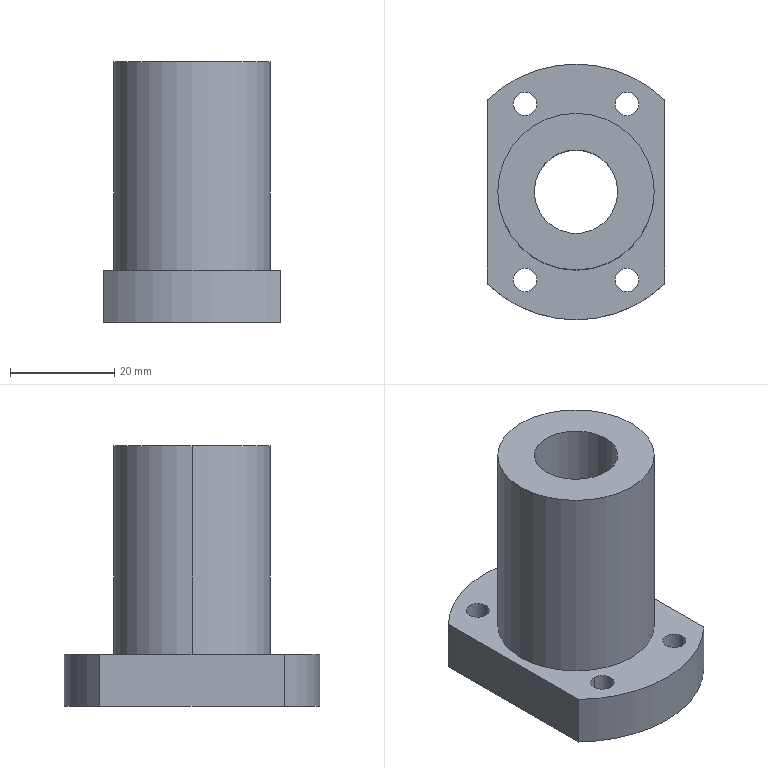Part | STEP file | SFI1605-4 | 2 solids | 34 faces | box 34 x 49 x 50 mm | volume 32157 mm3 | cylinder 24 | plane 10 | commonest cylinder face diameters 4.5 x8 8 x8 16 x4 30 x2 49 x2
STEP:
#1=CARTESIAN_POINT('',(8.,0.,523.5));
#2=VERTEX_POINT('',#1);
#3=CARTESIAN_POINT('',(-8.,0.,523.5));
#4=VERTEX_POINT('',#3);
#5=CARTESIAN_POINT('',(0.,0.,523.5));
#6=DIRECTION('',(0.,0.,-1.));
#7=DIRECTION('',(1.,0.,0.));
#8=AXIS2_PLACEMENT_3D('',#5,#6,#7);
#9=CIRCLE('',#8,8.);
#10=EDGE_CURVE('',#2,#4,#9,.T.);
#11=ORIENTED_EDGE('',*,*,#10,.F.);
#12=CARTESIAN_POINT('',(8.,0.,483.5));
#13=VERTEX_POINT('',#12);
#14=CARTESIAN_POINT('',(8.,0.,523.5));
#15=DIRECTION('',(0.,0.,-1.));
#16=VECTOR('',#15,1000.);
#17=LINE('',#14,#16);
#18=EDGE_CURVE('',#2,#13,#17,.T.);
#19=ORIENTED_EDGE('',*,*,#18,.T.);
#20=CARTESIAN_POINT('',(-8.,0.,483.5));
#21=VERTEX_POINT('',#20);
#22=CARTESIAN_POINT('',(0.,0.,483.5));
#23=DIRECTION('',(0.,0.,1.));
#24=DIRECTION('',(1.,0.,0.));
#25=AXIS2_PLACEMENT_3D('',#22,#23,#24);
#26=CIRCLE('',#25,8.);
#27=EDGE_CURVE('',#21,#13,#26,.T.);
#28=ORIENTED_EDGE('',*,*,#27,.F.);
#29=CARTESIAN_POINT('',(-8.,0.,523.5));
#30=DIRECTION('',(0.,0.,-1.));
#31=VECTOR('',#30,1000.);
#32=LINE('',#29,#31);
#33=EDGE_CURVE('',#4,#21,#32,.T.);
#34=ORIENTED_EDGE('',*,*,#33,.F.);
#35=EDGE_LOOP('',(#11,#19,#28,#34));
#36=FACE_OUTER_BOUND('',#35,.T.);
#37=CARTESIAN_POINT('',(0.,0.,523.5));
#38=DIRECTION('',(0.,0.,-1.));
#39=DIRECTION('',(-1.,0.,0.));
#40=AXIS2_PLACEMENT_3D('',#37,#38,#39);
#41=CYLINDRICAL_SURFACE('',#40,8.);
#42=ADVANCED_FACE('',(#36),#41,.F.);
#43=CARTESIAN_POINT('',(-15.,0.,523.5));
#44=VERTEX_POINT('',#43);
#45=CARTESIAN_POINT('',(15.,0.,523.5));
#46=VERTEX_POINT('',#45);
#47=CARTESIAN_POINT('',(0.,0.,523.5));
#48=DIRECTION('',(0.,0.,-1.));
#49=DIRECTION('',(-1.,0.,0.));
#50=AXIS2_PLACEMENT_3D('',#47,#48,#49);
#51=CIRCLE('',#50,15.);
#52=EDGE_CURVE('',#44,#46,#51,.T.);
#53=ORIENTED_EDGE('',*,*,#52,.T.);
#54=CARTESIAN_POINT('',(15.,0.,483.5));
#55=VERTEX_POINT('',#54);
#56=CARTESIAN_POINT('',(15.,0.,483.5));
#57=DIRECTION('',(0.,0.,-1.));
#58=VECTOR('',#57,1000.);
#59=LINE('',#56,#58);
#60=EDGE_CURVE('',#46,#55,#59,.T.);
#61=ORIENTED_EDGE('',*,*,#60,.T.);
#62=CARTESIAN_POINT('',(-15.,0.,483.5));
#63=VERTEX_POINT('',#62);
#64=CARTESIAN_POINT('',(0.,0.,483.5));
#65=DIRECTION('',(0.,0.,-1.));
#66=DIRECTION('',(-1.,0.,0.));
#67=AXIS2_PLACEMENT_3D('',#64,#65,#66);
#68=CIRCLE('',#67,15.);
#69=EDGE_CURVE('',#63,#55,#68,.T.);
#70=ORIENTED_EDGE('',*,*,#69,.F.);
#71=CARTESIAN_POINT('',(-15.,0.,483.5));
#72=DIRECTION('',(0.,0.,-1.));
#73=VECTOR('',#72,1000.);
#74=LINE('',#71,#73);
#75=EDGE_CURVE('',#44,#63,#74,.T.);
#76=ORIENTED_EDGE('',*,*,#75,.F.);
#77=EDGE_LOOP('',(#53,#61,#70,#76));
#78=FACE_OUTER_BOUND('',#77,.T.);
#79=CARTESIAN_POINT('',(0.,0.,483.5));
#80=DIRECTION('',(0.,0.,-1.));
#81=DIRECTION('',(-1.,0.,0.));
#82=AXIS2_PLACEMENT_3D('',#79,#80,#81);
#83=CYLINDRICAL_SURFACE('',#82,15.);
#84=ADVANCED_FACE('',(#78),#83,.T.);
#85=ORIENTED_EDGE('',*,*,#60,.F.);
#86=CARTESIAN_POINT('',(0.,0.,523.5));
#87=DIRECTION('',(0.,0.,-1.));
#88=DIRECTION('',(-1.,0.,0.));
#89=AXIS2_PLACEMENT_3D('',#86,#87,#88);
#90=CIRCLE('',#89,15.);
#91=EDGE_CURVE('',#46,#44,#90,.T.);
#92=ORIENTED_EDGE('',*,*,#91,.T.);
#93=ORIENTED_EDGE('',*,*,#75,.T.);
#94=CARTESIAN_POINT('',(0.,0.,483.5));
#95=DIRECTION('',(0.,0.,-1.));
#96=DIRECTION('',(-1.,0.,0.));
#97=AXIS2_PLACEMENT_3D('',#94,#95,#96);
#98=CIRCLE('',#97,15.);
#99=EDGE_CURVE('',#55,#63,#98,.T.);
#100=ORIENTED_EDGE('',*,*,#99,.F.);
#101=EDGE_LOOP('',(#85,#92,#93,#100));
#102=FACE_OUTER_BOUND('',#101,.T.);
#103=CARTESIAN_POINT('',(0.,0.,483.5));
#104=DIRECTION('',(0.,0.,-1.));
#105=DIRECTION('',(-1.,0.,0.));
#106=AXIS2_PLACEMENT_3D('',#103,#104,#105);
#107=CYLINDRICAL_SURFACE('',#106,15.);
#108=ADVANCED_FACE('',(#102),#107,.T.);
#109=ORIENTED_EDGE('',*,*,#27,.T.);
#110=CARTESIAN_POINT('',(0.,0.,483.5));
#111=DIRECTION('',(0.,0.,1.));
#112=DIRECTION('',(1.,0.,0.));
#113=AXIS2_PLACEMENT_3D('',#110,#111,#112);
#114=CIRCLE('',#113,8.);
#115=EDGE_CURVE('',#13,#21,#114,.T.);
#116=ORIENTED_EDGE('',*,*,#115,.T.);
#117=EDGE_LOOP('',(#109,#116));
#118=FACE_BOUND('',#117,.T.);
#119=ORIENTED_EDGE('',*,*,#69,.T.);
#120=ORIENTED_EDGE('',*,*,#99,.T.);
#121=EDGE_LOOP('',(#119,#120));
#122=FACE_OUTER_BOUND('',#121,.T.);
#123=CARTESIAN_POINT('',(15.,0.,483.5));
#124=DIRECTION('',(0.,0.,1.));
#125=DIRECTION('',(1.,0.,0.));
#126=AXIS2_PLACEMENT_3D('',#123,#124,#125);
#127=PLANE('',#126);
#128=ADVANCED_FACE('',(#118,#122),#127,.F.);
#129=CARTESIAN_POINT('',(0.,0.,523.5));
#130=DIRECTION('',(0.,0.,-1.));
#131=DIRECTION('',(1.,0.,0.));
#132=AXIS2_PLACEMENT_3D('',#129,#130,#131);
#133=CIRCLE('',#132,8.);
#134=EDGE_CURVE('',#4,#2,#133,.T.);
#135=ORIENTED_EDGE('',*,*,#134,.T.);
#136=ORIENTED_EDGE('',*,*,#10,.T.);
#137=EDGE_LOOP('',(#135,#136));
#138=FACE_BOUND('',#137,.T.);
#139=ORIENTED_EDGE('',*,*,#52,.F.);
#140=ORIENTED_EDGE('',*,*,#91,.F.);
#141=EDGE_LOOP('',(#139,#140));
#142=FACE_OUTER_BOUND('',#141,.T.);
#143=CARTESIAN_POINT('',(0.,0.,523.5));
#144=DIRECTION('',(0.,0.,-1.));
#145=DIRECTION('',(-1.,0.,0.));
#146=AXIS2_PLACEMENT_3D('',#143,#144,#145);
#147=PLANE('',#146);
#148=ADVANCED_FACE('',(#138,#142),#147,.F.);
#149=ORIENTED_EDGE('',*,*,#18,.F.);
#150=ORIENTED_EDGE('',*,*,#134,.F.);
#151=ORIENTED_EDGE('',*,*,#33,.T.);
#152=ORIENTED_EDGE('',*,*,#115,.F.);
#153=EDGE_LOOP('',(#149,#150,#151,#152));
#154=FACE_OUTER_BOUND('',#153,.T.);
#155=CARTESIAN_POINT('',(0.,0.,523.5));
#156=DIRECTION('',(0.,0.,-1.));
#157=DIRECTION('',(-1.,0.,0.));
#158=AXIS2_PLACEMENT_3D('',#155,#156,#157);
#159=CYLINDRICAL_SURFACE('',#158,8.);
#160=ADVANCED_FACE('',(#154),#159,.F.);
#161=CLOSED_SHELL('',(#42,#84,#108,#128,#148,#160));
#162=MANIFOLD_SOLID_BREP('',#161);
#163=CARTESIAN_POINT('',(-9.75,-20.887,478.1));
#164=VERTEX_POINT('',#163);
#165=CARTESIAN_POINT('',(-9.75,-12.887,478.1));
#166=VERTEX_POINT('',#165);
#167=CARTESIAN_POINT('',(-9.75,-16.887,478.1));
#168=DIRECTION('',(0.,0.,-1.));
#169=DIRECTION('',(0.,1.,0.));
#170=AXIS2_PLACEMENT_3D('',#167,#168,#169);
#171=CIRCLE('',#170,4.);
#172=EDGE_CURVE('',#164,#166,#171,.T.);
#173=ORIENTED_EDGE('',*,*,#172,.F.);
#174=CARTESIAN_POINT('',(-9.75,-20.887,473.5));
#175=VERTEX_POINT('',#174);
#176=CARTESIAN_POINT('',(-9.75,-20.887,473.5));
#177=DIRECTION('',(0.,0.,-1.));
#178=VECTOR('',#177,1000.);
#179=LINE('',#176,#178);
#180=EDGE_CURVE('',#164,#175,#179,.T.);
#181=ORIENTED_EDGE('',*,*,#180,.T.);
#182=CARTESIAN_POINT('',(-9.75,-12.887,473.5));
#183=VERTEX_POINT('',#182);
#184=CARTESIAN_POINT('',(-9.75,-16.887,473.5));
#185=DIRECTION('',(0.,0.,-1.));
#186=DIRECTION('',(0.,1.,0.));
#187=AXIS2_PLACEMENT_3D('',#184,#185,#186);
#188=CIRCLE('',#187,4.);
#189=EDGE_CURVE('',#175,#183,#188,.T.);
#190=ORIENTED_EDGE('',*,*,#189,.T.);
#191=CARTESIAN_POINT('',(-9.75,-12.887,473.5));
#192=DIRECTION('',(0.,0.,-1.));
#193=VECTOR('',#192,1000.);
#194=LINE('',#191,#193);
#195=EDGE_CURVE('',#166,#183,#194,.T.);
#196=ORIENTED_EDGE('',*,*,#195,.F.);
#197=EDGE_LOOP('',(#173,#181,#190,#196));
#198=FACE_OUTER_BOUND('',#197,.T.);
#199=CARTESIAN_POINT('',(-9.75,-16.887,473.5));
#200=DIRECTION('',(0.,0.,-1.));
#201=DIRECTION('',(0.,1.,0.));
#202=AXIS2_PLACEMENT_3D('',#199,#200,#201);
#203=CYLINDRICAL_SURFACE('',#202,4.);
#204=ADVANCED_FACE('',(#198),#203,.F.);
#205=CARTESIAN_POINT('',(-9.75,-19.137,483.5));
#206=VERTEX_POINT('',#205);
#207=CARTESIAN_POINT('',(-9.75,-14.637,483.5));
#208=VERTEX_POINT('',#207);
#209=CARTESIAN_POINT('',(-9.75,-16.887,483.5));
#210=DIRECTION('',(0.,0.,-1.));
#211=DIRECTION('',(0.,1.,0.));
#212=AXIS2_PLACEMENT_3D('',#209,#210,#211);
#213=CIRCLE('',#212,2.25);
#214=EDGE_CURVE('',#206,#208,#213,.T.);
#215=ORIENTED_EDGE('',*,*,#214,.F.);
#216=CARTESIAN_POINT('',(-9.75,-19.137,478.1));
#217=VERTEX_POINT('',#216);
#218=CARTESIAN_POINT('',(-9.75,-19.137,473.5));
#219=DIRECTION('',(0.,0.,-1.));
#220=VECTOR('',#219,1000.);
#221=LINE('',#218,#220);
#222=EDGE_CURVE('',#206,#217,#221,.T.);
#223=ORIENTED_EDGE('',*,*,#222,.T.);
#224=CARTESIAN_POINT('',(-9.75,-14.637,478.1));
#225=VERTEX_POINT('',#224);
#226=CARTESIAN_POINT('',(-9.75,-16.887,478.1));
#227=DIRECTION('',(0.,0.,-1.));
#228=DIRECTION('',(0.,1.,0.));
#229=AXIS2_PLACEMENT_3D('',#226,#227,#228);
#230=CIRCLE('',#229,2.25);
#231=EDGE_CURVE('',#217,#225,#230,.T.);
#232=ORIENTED_EDGE('',*,*,#231,.T.);
#233=CARTESIAN_POINT('',(-9.75,-14.637,473.5));
#234=DIRECTION('',(0.,0.,-1.));
#235=VECTOR('',#234,1000.);
#236=LINE('',#233,#235);
#237=EDGE_CURVE('',#208,#225,#236,.T.);
#238=ORIENTED_EDGE('',*,*,#237,.F.);
#239=EDGE_LOOP('',(#215,#223,#232,#238));
#240=FACE_OUTER_BOUND('',#239,.T.);
#241=CARTESIAN_POINT('',(-9.75,-16.887,473.5));
#242=DIRECTION('',(0.,0.,-1.));
#243=DIRECTION('',(0.,1.,0.));
#244=AXIS2_PLACEMENT_3D('',#241,#242,#243);
#245=CYLINDRICAL_SURFACE('',#244,2.25);
#246=ADVANCED_FACE('',(#240),#245,.F.);
#247=CARTESIAN_POINT('',(13.75,-16.887,478.1));
#248=VERTEX_POINT('',#247);
#249=CARTESIAN_POINT('',(5.75,-16.887,478.1));
#250=VERTEX_POINT('',#249);
#251=CARTESIAN_POINT('',(9.75,-16.887,478.1));
#252=DIRECTION('',(0.,0.,-1.));
#253=DIRECTION('',(-1.,0.,0.));
#254=AXIS2_PLACEMENT_3D('',#251,#252,#253);
#255=CIRCLE('',#254,4.);
#256=EDGE_CURVE('',#248,#250,#255,.T.);
#257=ORIENTED_EDGE('',*,*,#256,.F.);
#258=CARTESIAN_POINT('',(13.75,-16.887,473.5));
#259=VERTEX_POINT('',#258);
#260=CARTESIAN_POINT('',(13.75,-16.887,473.5));
#261=DIRECTION('',(0.,0.,-1.));
#262=VECTOR('',#261,1000.);
#263=LINE('',#260,#262);
#264=EDGE_CURVE('',#248,#259,#263,.T.);
#265=ORIENTED_EDGE('',*,*,#264,.T.);
#266=CARTESIAN_POINT('',(5.75,-16.887,473.5));
#267=VERTEX_POINT('',#266);
#268=CARTESIAN_POINT('',(9.75,-16.887,473.5));
#269=DIRECTION('',(0.,0.,-1.));
#270=DIRECTION('',(-1.,0.,0.));
#271=AXIS2_PLACEMENT_3D('',#268,#269,#270);
#272=CIRCLE('',#271,4.);
#273=EDGE_CURVE('',#259,#267,#272,.T.);
#274=ORIENTED_EDGE('',*,*,#273,.T.);
#275=CARTESIAN_POINT('',(5.75,-16.887,473.5));
#276=DIRECTION('',(0.,0.,-1.));
#277=VECTOR('',#276,1000.);
#278=LINE('',#275,#277);
#279=EDGE_CURVE('',#250,#267,#278,.T.);
#280=ORIENTED_EDGE('',*,*,#279,.F.);
#281=EDGE_LOOP('',(#257,#265,#274,#280));
#282=FACE_OUTER_BOUND('',#281,.T.);
#283=CARTESIAN_POINT('',(9.75,-16.887,473.5));
#284=DIRECTION('',(0.,0.,-1.));
#285=DIRECTION('',(-1.,0.,0.));
#286=AXIS2_PLACEMENT_3D('',#283,#284,#285);
#287=CYLINDRICAL_SURFACE('',#286,4.);
#288=ADVANCED_FACE('',(#282),#287,.F.);
#289=CARTESIAN_POINT('',(12.,-16.887,483.5));
#290=VERTEX_POINT('',#289);
#291=CARTESIAN_POINT('',(7.5,-16.887,483.5));
#292=VERTEX_POINT('',#291);
#293=CARTESIAN_POINT('',(9.75,-16.887,483.5));
#294=DIRECTION('',(0.,0.,-1.));
#295=DIRECTION('',(-1.,0.,0.));
#296=AXIS2_PLACEMENT_3D('',#293,#294,#295);
#297=CIRCLE('',#296,2.25);
#298=EDGE_CURVE('',#290,#292,#297,.T.);
#299=ORIENTED_EDGE('',*,*,#298,.F.);
#300=CARTESIAN_POINT('',(12.,-16.887,478.1));
#301=VERTEX_POINT('',#300);
#302=CARTESIAN_POINT('',(12.,-16.887,473.5));
#303=DIRECTION('',(0.,0.,-1.));
#304=VECTOR('',#303,1000.);
#305=LINE('',#302,#304);
#306=EDGE_CURVE('',#290,#301,#305,.T.);
#307=ORIENTED_EDGE('',*,*,#306,.T.);
#308=CARTESIAN_POINT('',(7.5,-16.887,478.1));
#309=VERTEX_POINT('',#308);
#310=CARTESIAN_POINT('',(9.75,-16.887,478.1));
#311=DIRECTION('',(0.,0.,-1.));
#312=DIRECTION('',(-1.,0.,0.));
#313=AXIS2_PLACEMENT_3D('',#310,#311,#312);
#314=CIRCLE('',#313,2.25);
#315=EDGE_CURVE('',#301,#309,#314,.T.);
#316=ORIENTED_EDGE('',*,*,#315,.T.);
#317=CARTESIAN_POINT('',(7.5,-16.887,473.5));
#318=DIRECTION('',(0.,0.,-1.));
#319=VECTOR('',#318,1000.);
#320=LINE('',#317,#319);
#321=EDGE_CURVE('',#292,#309,#320,.T.);
#322=ORIENTED_EDGE('',*,*,#321,.F.);
#323=EDGE_LOOP('',(#299,#307,#316,#322));
#324=FACE_OUTER_BOUND('',#323,.T.);
#325=CARTESIAN_POINT('',(9.75,-16.887,473.5));
#326=DIRECTION('',(0.,0.,-1.));
#327=DIRECTION('',(-1.,0.,0.));
#328=AXIS2_PLACEMENT_3D('',#325,#326,#327);
#329=CYLINDRICAL_SURFACE('',#328,2.25);
#330=ADVANCED_FACE('',(#324),#329,.F.);
#331=CARTESIAN_POINT('',(9.75,12.887,478.1));
#332=VERTEX_POINT('',#331);
#333=CARTESIAN_POINT('',(9.75,20.887,478.1));
#334=VERTEX_POINT('',#333);
#335=CARTESIAN_POINT('',(9.75,16.887,478.1));
#336=DIRECTION('',(0.,0.,-1.));
#337=DIRECTION('',(0.,1.,0.));
#338=AXIS2_PLACEMENT_3D('',#335,#336,#337);
#339=CIRCLE('',#338,4.);
#340=EDGE_CURVE('',#332,#334,#339,.T.);
#341=ORIENTED_EDGE('',*,*,#340,.F.);
#342=CARTESIAN_POINT('',(9.75,12.887,473.5));
#343=VERTEX_POINT('',#342);
#344=CARTESIAN_POINT('',(9.75,12.887,473.5));
#345=DIRECTION('',(0.,0.,-1.));
#346=VECTOR('',#345,1000.);
#347=LINE('',#344,#346);
#348=EDGE_CURVE('',#332,#343,#347,.T.);
#349=ORIENTED_EDGE('',*,*,#348,.T.);
#350=CARTESIAN_POINT('',(9.75,20.887,473.5));
#351=VERTEX_POINT('',#350);
#352=CARTESIAN_POINT('',(9.75,16.887,473.5));
#353=DIRECTION('',(0.,0.,-1.));
#354=DIRECTION('',(0.,1.,0.));
#355=AXIS2_PLACEMENT_3D('',#352,#353,#354);
#356=CIRCLE('',#355,4.);
#357=EDGE_CURVE('',#343,#351,#356,.T.);
#358=ORIENTED_EDGE('',*,*,#357,.T.);
#359=CARTESIAN_POINT('',(9.75,20.887,473.5));
#360=DIRECTION('',(0.,0.,-1.));
#361=VECTOR('',#360,1000.);
#362=LINE('',#359,#361);
#363=EDGE_CURVE('',#334,#351,#362,.T.);
#364=ORIENTED_EDGE('',*,*,#363,.F.);
#365=EDGE_LOOP('',(#341,#349,#358,#364));
#366=FACE_OUTER_BOUND('',#365,.T.);
#367=CARTESIAN_POINT('',(9.75,16.887,473.5));
#368=DIRECTION('',(0.,0.,-1.));
#369=DIRECTION('',(0.,1.,0.));
#370=AXIS2_PLACEMENT_3D('',#367,#368,#369);
#371=CYLINDRICAL_SURFACE('',#370,4.);
#372=ADVANCED_FACE('',(#366),#371,.F.);
#373=CARTESIAN_POINT('',(9.75,14.637,483.5));
#374=VERTEX_POINT('',#373);
#375=CARTESIAN_POINT('',(9.75,19.137,483.5));
#376=VERTEX_POINT('',#375);
#377=CARTESIAN_POINT('',(9.75,16.887,483.5));
#378=DIRECTION('',(0.,0.,-1.));
#379=DIRECTION('',(0.,1.,0.));
#380=AXIS2_PLACEMENT_3D('',#377,#378,#379);
#381=CIRCLE('',#380,2.25);
#382=EDGE_CURVE('',#374,#376,#381,.T.);
#383=ORIENTED_EDGE('',*,*,#382,.F.);
#384=CARTESIAN_POINT('',(9.75,14.637,478.1));
#385=VERTEX_POINT('',#384);
#386=CARTESIAN_POINT('',(9.75,14.637,473.5));
#387=DIRECTION('',(0.,0.,-1.));
#388=VECTOR('',#387,1000.);
#389=LINE('',#386,#388);
#390=EDGE_CURVE('',#374,#385,#389,.T.);
#391=ORIENTED_EDGE('',*,*,#390,.T.);
#392=CARTESIAN_POINT('',(9.75,19.137,478.1));
#393=VERTEX_POINT('',#392);
#394=CARTESIAN_POINT('',(9.75,16.887,478.1));
#395=DIRECTION('',(0.,0.,-1.));
#396=DIRECTION('',(0.,1.,0.));
#397=AXIS2_PLACEMENT_3D('',#394,#395,#396);
#398=CIRCLE('',#397,2.25);
#399=EDGE_CURVE('',#385,#393,#398,.T.);
#400=ORIENTED_EDGE('',*,*,#399,.T.);
#401=CARTESIAN_POINT('',(9.75,19.137,473.5));
#402=DIRECTION('',(0.,0.,-1.));
#403=VECTOR('',#402,1000.);
#404=LINE('',#401,#403);
#405=EDGE_CURVE('',#376,#393,#404,.T.);
#406=ORIENTED_EDGE('',*,*,#405,.F.);
#407=EDGE_LOOP('',(#383,#391,#400,#406));
#408=FACE_OUTER_BOUND('',#407,.T.);
#409=CARTESIAN_POINT('',(9.75,16.887,473.5));
#410=DIRECTION('',(0.,0.,-1.));
#411=DIRECTION('',(0.,1.,0.));
#412=AXIS2_PLACEMENT_3D('',#409,#410,#411);
#413=CYLINDRICAL_SURFACE('',#412,2.25);
#414=ADVANCED_FACE('',(#408),#413,.F.);
#415=CARTESIAN_POINT('',(-5.75,16.887,478.1));
#416=VERTEX_POINT('',#415);
#417=CARTESIAN_POINT('',(-13.75,16.887,478.1));
#418=VERTEX_POINT('',#417);
#419=CARTESIAN_POINT('',(-9.75,16.887,478.1));
#420=DIRECTION('',(0.,0.,-1.));
#421=DIRECTION('',(-1.,0.,0.));
#422=AXIS2_PLACEMENT_3D('',#419,#420,#421);
#423=CIRCLE('',#422,4.);
#424=EDGE_CURVE('',#416,#418,#423,.T.);
#425=ORIENTED_EDGE('',*,*,#424,.F.);
#426=CARTESIAN_POINT('',(-5.75,16.887,473.5));
#427=VERTEX_POINT('',#426);
#428=CARTESIAN_POINT('',(-5.75,16.887,473.5));
#429=DIRECTION('',(0.,0.,-1.));
#430=VECTOR('',#429,1000.);
#431=LINE('',#428,#430);
#432=EDGE_CURVE('',#416,#427,#431,.T.);
#433=ORIENTED_EDGE('',*,*,#432,.T.);
#434=CARTESIAN_POINT('',(-13.75,16.887,473.5));
#435=VERTEX_POINT('',#434);
#436=CARTESIAN_POINT('',(-9.75,16.887,473.5));
#437=DIRECTION('',(0.,0.,-1.));
#438=DIRECTION('',(-1.,0.,0.));
#439=AXIS2_PLACEMENT_3D('',#436,#437,#438);
#440=CIRCLE('',#439,4.);
#441=EDGE_CURVE('',#427,#435,#440,.T.);
#442=ORIENTED_EDGE('',*,*,#441,.T.);
#443=CARTESIAN_POINT('',(-13.75,16.887,473.5));
#444=DIRECTION('',(0.,0.,-1.));
#445=VECTOR('',#444,1000.);
#446=LINE('',#443,#445);
#447=EDGE_CURVE('',#418,#435,#446,.T.);
#448=ORIENTED_EDGE('',*,*,#447,.F.);
#449=EDGE_LOOP('',(#425,#433,#442,#448));
#450=FACE_OUTER_BOUND('',#449,.T.);
#451=CARTESIAN_POINT('',(-9.75,16.887,473.5));
#452=DIRECTION('',(0.,0.,-1.));
#453=DIRECTION('',(-1.,0.,0.));
#454=AXIS2_PLACEMENT_3D('',#451,#452,#453);
#455=CYLINDRICAL_SURFACE('',#454,4.);
#456=ADVANCED_FACE('',(#450),#455,.F.);
#457=CARTESIAN_POINT('',(-7.5,16.887,483.5));
#458=VERTEX_POINT('',#457);
#459=CARTESIAN_POINT('',(-12.,16.887,483.5));
#460=VERTEX_POINT('',#459);
#461=CARTESIAN_POINT('',(-9.75,16.887,483.5));
#462=DIRECTION('',(0.,0.,-1.));
#463=DIRECTION('',(-1.,0.,0.));
#464=AXIS2_PLACEMENT_3D('',#461,#462,#463);
#465=CIRCLE('',#464,2.25);
#466=EDGE_CURVE('',#458,#460,#465,.T.);
#467=ORIENTED_EDGE('',*,*,#466,.F.);
#468=CARTESIAN_POINT('',(-7.5,16.887,478.1));
#469=VERTEX_POINT('',#468);
#470=CARTESIAN_POINT('',(-7.5,16.887,473.5));
#471=DIRECTION('',(0.,0.,-1.));
#472=VECTOR('',#471,1000.);
#473=LINE('',#470,#472);
#474=EDGE_CURVE('',#458,#469,#473,.T.);
#475=ORIENTED_EDGE('',*,*,#474,.T.);
#476=CARTESIAN_POINT('',(-12.,16.887,478.1));
#477=VERTEX_POINT('',#476);
#478=CARTESIAN_POINT('',(-9.75,16.887,478.1));
#479=DIRECTION('',(0.,0.,-1.));
#480=DIRECTION('',(-1.,0.,0.));
#481=AXIS2_PLACEMENT_3D('',#478,#479,#480);
#482=CIRCLE('',#481,2.25);
#483=EDGE_CURVE('',#469,#477,#482,.T.);
#484=ORIENTED_EDGE('',*,*,#483,.T.);
#485=CARTESIAN_POINT('',(-12.,16.887,473.5));
#486=DIRECTION('',(0.,0.,-1.));
#487=VECTOR('',#486,1000.);
#488=LINE('',#485,#487);
#489=EDGE_CURVE('',#460,#477,#488,.T.);
#490=ORIENTED_EDGE('',*,*,#489,.F.);
#491=EDGE_LOOP('',(#467,#475,#484,#490));
#492=FACE_OUTER_BOUND('',#491,.T.);
#493=CARTESIAN_POINT('',(-9.75,16.887,473.5));
#494=DIRECTION('',(0.,0.,-1.));
#495=DIRECTION('',(-1.,0.,0.));
#496=AXIS2_PLACEMENT_3D('',#493,#494,#495);
#497=CYLINDRICAL_SURFACE('',#496,2.25);
#498=ADVANCED_FACE('',(#492),#497,.F.);
#499=CARTESIAN_POINT('',(8.,0.,483.5));
#500=VERTEX_POINT('',#499);
#501=CARTESIAN_POINT('',(-8.,0.,483.5));
#502=VERTEX_POINT('',#501);
#503=CARTESIAN_POINT('',(0.,0.,483.5));
#504=DIRECTION('',(0.,0.,-1.));
#505=DIRECTION('',(-1.,0.,0.));
#506=AXIS2_PLACEMENT_3D('',#503,#504,#505);
#507=CIRCLE('',#506,8.);
#508=EDGE_CURVE('',#500,#502,#507,.T.);
#509=ORIENTED_EDGE('',*,*,#508,.F.);
#510=CARTESIAN_POINT('',(8.,0.,473.5));
#511=VERTEX_POINT('',#510);
#512=CARTESIAN_POINT('',(8.,0.,523.5));
#513=DIRECTION('',(0.,0.,-1.));
#514=VECTOR('',#513,1000.);
#515=LINE('',#512,#514);
#516=EDGE_CURVE('',#500,#511,#515,.T.);
#517=ORIENTED_EDGE('',*,*,#516,.T.);
#518=CARTESIAN_POINT('',(-8.,0.,473.5));
#519=VERTEX_POINT('',#518);
#520=CARTESIAN_POINT('',(0.,0.,473.5));
#521=DIRECTION('',(0.,0.,-1.));
#522=DIRECTION('',(-1.,0.,0.));
#523=AXIS2_PLACEMENT_3D('',#520,#521,#522);
#524=CIRCLE('',#523,8.);
#525=EDGE_CURVE('',#511,#519,#524,.T.);
#526=ORIENTED_EDGE('',*,*,#525,.T.);
#527=CARTESIAN_POINT('',(-8.,0.,523.5));
#528=DIRECTION('',(0.,0.,-1.));
#529=VECTOR('',#528,1000.);
#530=LINE('',#527,#529);
#531=EDGE_CURVE('',#502,#519,#530,.T.);
#532=ORIENTED_EDGE('',*,*,#531,.F.);
#533=EDGE_LOOP('',(#509,#517,#526,#532));
#534=FACE_OUTER_BOUND('',#533,.T.);
#535=CARTESIAN_POINT('',(0.,0.,523.5));
#536=DIRECTION('',(0.,0.,-1.));
#537=DIRECTION('',(-1.,0.,0.));
#538=AXIS2_PLACEMENT_3D('',#535,#536,#537);
#539=CYLINDRICAL_SURFACE('',#538,8.);
#540=ADVANCED_FACE('',(#534),#539,.F.);
#541=CARTESIAN_POINT('',(-17.,17.642,483.5));
#542=VERTEX_POINT('',#541);
#543=CARTESIAN_POINT('',(17.,17.642,483.5));
#544=VERTEX_POINT('',#543);
#545=CARTESIAN_POINT('',(0.,0.,483.5));
#546=DIRECTION('',(0.,0.,-1.));
#547=DIRECTION('',(-1.,0.,0.));
#548=AXIS2_PLACEMENT_3D('',#545,#546,#547);
#549=CIRCLE('',#548,24.5);
#550=EDGE_CURVE('',#542,#544,#549,.T.);
#551=ORIENTED_EDGE('',*,*,#550,.T.);
#552=CARTESIAN_POINT('',(17.,17.642,473.5));
#553=VERTEX_POINT('',#552);
#554=CARTESIAN_POINT('',(17.,17.642,473.5));
#555=DIRECTION('',(0.,0.,1.));
#556=VECTOR('',#555,1000.);
#557=LINE('',#554,#556);
#558=EDGE_CURVE('',#553,#544,#557,.T.);
#559=ORIENTED_EDGE('',*,*,#558,.F.);
#560=CARTESIAN_POINT('',(-17.,17.642,473.5));
#561=VERTEX_POINT('',#560);
#562=CARTESIAN_POINT('',(0.,0.,473.5));
#563=DIRECTION('',(0.,0.,-1.));
#564=DIRECTION('',(-1.,0.,0.));
#565=AXIS2_PLACEMENT_3D('',#562,#563,#564);
#566=CIRCLE('',#565,24.5);
#567=EDGE_CURVE('',#561,#553,#566,.T.);
#568=ORIENTED_EDGE('',*,*,#567,.F.);
#569=CARTESIAN_POINT('',(-17.,17.642,473.5));
#570=DIRECTION('',(0.,0.,1.));
#571=VECTOR('',#570,1000.);
#572=LINE('',#569,#571);
#573=EDGE_CURVE('',#561,#542,#572,.T.);
#574=ORIENTED_EDGE('',*,*,#573,.T.);
#575=EDGE_LOOP('',(#551,#559,#568,#574));
#576=FACE_OUTER_BOUND('',#575,.T.);
#577=CARTESIAN_POINT('',(0.,0.,473.5));
#578=DIRECTION('',(0.,0.,1.));
#579=DIRECTION('',(1.,0.,0.));
#580=AXIS2_PLACEMENT_3D('',#577,#578,#579);
#581=CYLINDRICAL_SURFACE('',#580,24.5);
#582=ADVANCED_FACE('',(#576),#581,.T.);
#583=CARTESIAN_POINT('',(17.,-17.642,483.5));
#584=VERTEX_POINT('',#583);
#585=CARTESIAN_POINT('',(17.,17.642,483.5));
#586=DIRECTION('',(0.,-1.,0.));
#587=VECTOR('',#586,1000.);
#588=LINE('',#585,#587);
#589=EDGE_CURVE('',#544,#584,#588,.T.);
#590=ORIENTED_EDGE('',*,*,#589,.T.);
#591=CARTESIAN_POINT('',(17.,-17.642,473.5));
#592=VERTEX_POINT('',#591);
#593=CARTESIAN_POINT('',(17.,-17.642,473.5));
#594=DIRECTION('',(0.,0.,1.));
#595=VECTOR('',#594,1000.);
#596=LINE('',#593,#595);
#597=EDGE_CURVE('',#592,#584,#596,.T.);
#598=ORIENTED_EDGE('',*,*,#597,.F.);
#599=CARTESIAN_POINT('',(17.,17.642,473.5));
#600=DIRECTION('',(0.,-1.,0.));
#601=VECTOR('',#600,1000.);
#602=LINE('',#599,#601);
#603=EDGE_CURVE('',#553,#592,#602,.T.);
#604=ORIENTED_EDGE('',*,*,#603,.F.);
#605=ORIENTED_EDGE('',*,*,#558,.T.);
#606=EDGE_LOOP('',(#590,#598,#604,#605));
#607=FACE_OUTER_BOUND('',#606,.T.);
#608=CARTESIAN_POINT('',(17.,17.642,473.5));
#609=DIRECTION('',(-1.,0.,0.));
#610=DIRECTION('',(0.,0.,1.));
#611=AXIS2_PLACEMENT_3D('',#608,#609,#610);
#612=PLANE('',#611);
#613=ADVANCED_FACE('',(#607),#612,.F.);
#614=CARTESIAN_POINT('',(-17.,-17.642,483.5));
#615=VERTEX_POINT('',#614);
#616=CARTESIAN_POINT('',(0.,0.,483.5));
#617=DIRECTION('',(0.,0.,-1.));
#618=DIRECTION('',(-1.,0.,0.));
#619=AXIS2_PLACEMENT_3D('',#616,#617,#618);
#620=CIRCLE('',#619,24.5);
#621=EDGE_CURVE('',#584,#615,#620,.T.);
#622=ORIENTED_EDGE('',*,*,#621,.T.);
#623=CARTESIAN_POINT('',(-17.,-17.642,473.5));
#624=VERTEX_POINT('',#623);
#625=CARTESIAN_POINT('',(-17.,-17.642,473.5));
#626=DIRECTION('',(0.,0.,1.));
#627=VECTOR('',#626,1000.);
#628=LINE('',#625,#627);
#629=EDGE_CURVE('',#624,#615,#628,.T.);
#630=ORIENTED_EDGE('',*,*,#629,.F.);
#631=CARTESIAN_POINT('',(0.,0.,473.5));
#632=DIRECTION('',(0.,0.,-1.));
#633=DIRECTION('',(-1.,0.,0.));
#634=AXIS2_PLACEMENT_3D('',#631,#632,#633);
#635=CIRCLE('',#634,24.5);
#636=EDGE_CURVE('',#592,#624,#635,.T.);
#637=ORIENTED_EDGE('',*,*,#636,.F.);
#638=ORIENTED_EDGE('',*,*,#597,.T.);
#639=EDGE_LOOP('',(#622,#630,#637,#638));
#640=FACE_OUTER_BOUND('',#639,.T.);
#641=CARTESIAN_POINT('',(0.,0.,473.5));
#642=DIRECTION('',(0.,0.,1.));
#643=DIRECTION('',(1.,0.,0.));
#644=AXIS2_PLACEMENT_3D('',#641,#642,#643);
#645=CYLINDRICAL_SURFACE('',#644,24.5);
#646=ADVANCED_FACE('',(#640),#645,.T.);
#647=CARTESIAN_POINT('',(-17.,-17.642,483.5));
#648=DIRECTION('',(0.,1.,0.));
#649=VECTOR('',#648,1000.);
#650=LINE('',#647,#649);
#651=EDGE_CURVE('',#615,#542,#650,.T.);
#652=ORIENTED_EDGE('',*,*,#651,.T.);
#653=ORIENTED_EDGE('',*,*,#573,.F.);
#654=CARTESIAN_POINT('',(-17.,-17.642,473.5));
#655=DIRECTION('',(0.,1.,0.));
#656=VECTOR('',#655,1000.);
#657=LINE('',#654,#656);
#658=EDGE_CURVE('',#624,#561,#657,.T.);
#659=ORIENTED_EDGE('',*,*,#658,.F.);
#660=ORIENTED_EDGE('',*,*,#629,.T.);
#661=EDGE_LOOP('',(#652,#653,#659,#660));
#662=FACE_OUTER_BOUND('',#661,.T.);
#663=CARTESIAN_POINT('',(-17.,-17.642,473.5));
#664=DIRECTION('',(1.,0.,0.));
#665=DIRECTION('',(0.,0.,-1.));
#666=AXIS2_PLACEMENT_3D('',#663,#664,#665);
#667=PLANE('',#666);
#668=ADVANCED_FACE('',(#662),#667,.F.);
#669=CARTESIAN_POINT('',(-9.75,-16.887,473.5));
#670=DIRECTION('',(0.,0.,-1.));
#671=DIRECTION('',(0.,1.,0.));
#672=AXIS2_PLACEMENT_3D('',#669,#670,#671);
#673=CIRCLE('',#672,4.);
#674=EDGE_CURVE('',#183,#175,#673,.T.);
#675=ORIENTED_EDGE('',*,*,#674,.F.);
#676=ORIENTED_EDGE('',*,*,#189,.F.);
#677=EDGE_LOOP('',(#675,#676));
#678=FACE_BOUND('',#677,.T.);
#679=CARTESIAN_POINT('',(9.75,-16.887,473.5));
#680=DIRECTION('',(0.,0.,-1.));
#681=DIRECTION('',(-1.,0.,0.));
#682=AXIS2_PLACEMENT_3D('',#679,#680,#681);
#683=CIRCLE('',#682,4.);
#684=EDGE_CURVE('',#267,#259,#683,.T.);
#685=ORIENTED_EDGE('',*,*,#684,.F.);
#686=ORIENTED_EDGE('',*,*,#273,.F.);
#687=EDGE_LOOP('',(#685,#686));
#688=FACE_BOUND('',#687,.T.);
#689=CARTESIAN_POINT('',(9.75,16.887,473.5));
#690=DIRECTION('',(0.,0.,-1.));
#691=DIRECTION('',(0.,1.,0.));
#692=AXIS2_PLACEMENT_3D('',#689,#690,#691);
#693=CIRCLE('',#692,4.);
#694=EDGE_CURVE('',#351,#343,#693,.T.);
#695=ORIENTED_EDGE('',*,*,#694,.F.);
#696=ORIENTED_EDGE('',*,*,#357,.F.);
#697=EDGE_LOOP('',(#695,#696));
#698=FACE_BOUND('',#697,.T.);
#699=CARTESIAN_POINT('',(-9.75,16.887,473.5));
#700=DIRECTION('',(0.,0.,-1.));
#701=DIRECTION('',(-1.,0.,0.));
#702=AXIS2_PLACEMENT_3D('',#699,#700,#701);
#703=CIRCLE('',#702,4.);
#704=EDGE_CURVE('',#435,#427,#703,.T.);
#705=ORIENTED_EDGE('',*,*,#704,.F.);
#706=ORIENTED_EDGE('',*,*,#441,.F.);
#707=EDGE_LOOP('',(#705,#706));
#708=FACE_BOUND('',#707,.T.);
#709=CARTESIAN_POINT('',(0.,0.,473.5));
#710=DIRECTION('',(0.,0.,-1.));
#711=DIRECTION('',(-1.,0.,0.));
#712=AXIS2_PLACEMENT_3D('',#709,#710,#711);
#713=CIRCLE('',#712,8.);
#714=EDGE_CURVE('',#519,#511,#713,.T.);
#715=ORIENTED_EDGE('',*,*,#714,.F.);
#716=ORIENTED_EDGE('',*,*,#525,.F.);
#717=EDGE_LOOP('',(#715,#716));
#718=FACE_BOUND('',#717,.T.);
#719=ORIENTED_EDGE('',*,*,#567,.T.);
#720=ORIENTED_EDGE('',*,*,#603,.T.);
#721=ORIENTED_EDGE('',*,*,#636,.T.);
#722=ORIENTED_EDGE('',*,*,#658,.T.);
#723=EDGE_LOOP('',(#719,#720,#721,#722));
#724=FACE_OUTER_BOUND('',#723,.T.);
#725=CARTESIAN_POINT('',(0.,0.,473.5));
#726=DIRECTION('',(0.,0.,-1.));
#727=DIRECTION('',(-1.,0.,0.));
#728=AXIS2_PLACEMENT_3D('',#725,#726,#727);
#729=PLANE('',#728);
#730=ADVANCED_FACE('',(#678,#688,#698,#708,#718,#724),#729,.T.);
#731=CARTESIAN_POINT('',(-9.75,-16.887,483.5));
#732=DIRECTION('',(0.,0.,-1.));
#733=DIRECTION('',(0.,1.,0.));
#734=AXIS2_PLACEMENT_3D('',#731,#732,#733);
#735=CIRCLE('',#734,2.25);
#736=EDGE_CURVE('',#208,#206,#735,.T.);
#737=ORIENTED_EDGE('',*,*,#736,.T.);
#738=ORIENTED_EDGE('',*,*,#214,.T.);
#739=EDGE_LOOP('',(#737,#738));
#740=FACE_BOUND('',#739,.T.);
#741=CARTESIAN_POINT('',(9.75,-16.887,483.5));
#742=DIRECTION('',(0.,0.,-1.));
#743=DIRECTION('',(-1.,0.,0.));
#744=AXIS2_PLACEMENT_3D('',#741,#742,#743);
#745=CIRCLE('',#744,2.25);
#746=EDGE_CURVE('',#292,#290,#745,.T.);
#747=ORIENTED_EDGE('',*,*,#746,.T.);
#748=ORIENTED_EDGE('',*,*,#298,.T.);
#749=EDGE_LOOP('',(#747,#748));
#750=FACE_BOUND('',#749,.T.);
#751=CARTESIAN_POINT('',(9.75,16.887,483.5));
#752=DIRECTION('',(0.,0.,-1.));
#753=DIRECTION('',(0.,1.,0.));
#754=AXIS2_PLACEMENT_3D('',#751,#752,#753);
#755=CIRCLE('',#754,2.25);
#756=EDGE_CURVE('',#376,#374,#755,.T.);
#757=ORIENTED_EDGE('',*,*,#756,.T.);
#758=ORIENTED_EDGE('',*,*,#382,.T.);
#759=EDGE_LOOP('',(#757,#758));
#760=FACE_BOUND('',#759,.T.);
#761=CARTESIAN_POINT('',(-9.75,16.887,483.5));
#762=DIRECTION('',(0.,0.,-1.));
#763=DIRECTION('',(-1.,0.,0.));
#764=AXIS2_PLACEMENT_3D('',#761,#762,#763);
#765=CIRCLE('',#764,2.25);
#766=EDGE_CURVE('',#460,#458,#765,.T.);
#767=ORIENTED_EDGE('',*,*,#766,.T.);
#768=ORIENTED_EDGE('',*,*,#466,.T.);
#769=EDGE_LOOP('',(#767,#768));
#770=FACE_BOUND('',#769,.T.);
#771=CARTESIAN_POINT('',(0.,0.,483.5));
#772=DIRECTION('',(0.,0.,-1.));
#773=DIRECTION('',(-1.,0.,0.));
#774=AXIS2_PLACEMENT_3D('',#771,#772,#773);
#775=CIRCLE('',#774,8.);
#776=EDGE_CURVE('',#502,#500,#775,.T.);
#777=ORIENTED_EDGE('',*,*,#776,.T.);
#778=ORIENTED_EDGE('',*,*,#508,.T.);
#779=EDGE_LOOP('',(#777,#778));
#780=FACE_BOUND('',#779,.T.);
#781=ORIENTED_EDGE('',*,*,#550,.F.);
#782=ORIENTED_EDGE('',*,*,#651,.F.);
#783=ORIENTED_EDGE('',*,*,#621,.F.);
#784=ORIENTED_EDGE('',*,*,#589,.F.);
#785=EDGE_LOOP('',(#781,#782,#783,#784));
#786=FACE_OUTER_BOUND('',#785,.T.);
#787=CARTESIAN_POINT('',(0.,0.,483.5));
#788=DIRECTION('',(0.,0.,-1.));
#789=DIRECTION('',(-1.,0.,0.));
#790=AXIS2_PLACEMENT_3D('',#787,#788,#789);
#791=PLANE('',#790);
#792=ADVANCED_FACE('',(#740,#750,#760,#770,#780,#786),#791,.F.);
#793=ORIENTED_EDGE('',*,*,#516,.F.);
#794=ORIENTED_EDGE('',*,*,#776,.F.);
#795=ORIENTED_EDGE('',*,*,#531,.T.);
#796=ORIENTED_EDGE('',*,*,#714,.T.);
#797=EDGE_LOOP('',(#793,#794,#795,#796));
#798=FACE_OUTER_BOUND('',#797,.T.);
#799=CARTESIAN_POINT('',(0.,0.,523.5));
#800=DIRECTION('',(0.,0.,-1.));
#801=DIRECTION('',(-1.,0.,0.));
#802=AXIS2_PLACEMENT_3D('',#799,#800,#801);
#803=CYLINDRICAL_SURFACE('',#802,8.);
#804=ADVANCED_FACE('',(#798),#803,.F.);
#805=ORIENTED_EDGE('',*,*,#474,.F.);
#806=ORIENTED_EDGE('',*,*,#766,.F.);
#807=ORIENTED_EDGE('',*,*,#489,.T.);
#808=CARTESIAN_POINT('',(-9.75,16.887,478.1));
#809=DIRECTION('',(0.,0.,-1.));
#810=DIRECTION('',(-1.,0.,0.));
#811=AXIS2_PLACEMENT_3D('',#808,#809,#810);
#812=CIRCLE('',#811,2.25);
#813=EDGE_CURVE('',#477,#469,#812,.T.);
#814=ORIENTED_EDGE('',*,*,#813,.T.);
#815=EDGE_LOOP('',(#805,#806,#807,#814));
#816=FACE_OUTER_BOUND('',#815,.T.);
#817=CARTESIAN_POINT('',(-9.75,16.887,473.5));
#818=DIRECTION('',(0.,0.,-1.));
#819=DIRECTION('',(-1.,0.,0.));
#820=AXIS2_PLACEMENT_3D('',#817,#818,#819);
#821=CYLINDRICAL_SURFACE('',#820,2.25);
#822=ADVANCED_FACE('',(#816),#821,.F.);
#823=ORIENTED_EDGE('',*,*,#813,.F.);
#824=ORIENTED_EDGE('',*,*,#483,.F.);
#825=EDGE_LOOP('',(#823,#824));
#826=FACE_BOUND('',#825,.T.);
#827=CARTESIAN_POINT('',(-9.75,16.887,478.1));
#828=DIRECTION('',(0.,0.,-1.));
#829=DIRECTION('',(-1.,0.,0.));
#830=AXIS2_PLACEMENT_3D('',#827,#828,#829);
#831=CIRCLE('',#830,4.);
#832=EDGE_CURVE('',#418,#416,#831,.T.);
#833=ORIENTED_EDGE('',*,*,#832,.T.);
#834=ORIENTED_EDGE('',*,*,#424,.T.);
#835=EDGE_LOOP('',(#833,#834));
#836=FACE_OUTER_BOUND('',#835,.T.);
#837=CARTESIAN_POINT('',(-7.5,16.887,478.1));
#838=DIRECTION('',(0.,0.,1.));
#839=DIRECTION('',(1.,0.,0.));
#840=AXIS2_PLACEMENT_3D('',#837,#838,#839);
#841=PLANE('',#840);
#842=ADVANCED_FACE('',(#826,#836),#841,.F.);
#843=ORIENTED_EDGE('',*,*,#432,.F.);
#844=ORIENTED_EDGE('',*,*,#832,.F.);
#845=ORIENTED_EDGE('',*,*,#447,.T.);
#846=ORIENTED_EDGE('',*,*,#704,.T.);
#847=EDGE_LOOP('',(#843,#844,#845,#846));
#848=FACE_OUTER_BOUND('',#847,.T.);
#849=CARTESIAN_POINT('',(-9.75,16.887,473.5));
#850=DIRECTION('',(0.,0.,-1.));
#851=DIRECTION('',(-1.,0.,0.));
#852=AXIS2_PLACEMENT_3D('',#849,#850,#851);
#853=CYLINDRICAL_SURFACE('',#852,4.);
#854=ADVANCED_FACE('',(#848),#853,.F.);
#855=ORIENTED_EDGE('',*,*,#390,.F.);
#856=ORIENTED_EDGE('',*,*,#756,.F.);
#857=ORIENTED_EDGE('',*,*,#405,.T.);
#858=CARTESIAN_POINT('',(9.75,16.887,478.1));
#859=DIRECTION('',(0.,0.,-1.));
#860=DIRECTION('',(0.,1.,0.));
#861=AXIS2_PLACEMENT_3D('',#858,#859,#860);
#862=CIRCLE('',#861,2.25);
#863=EDGE_CURVE('',#393,#385,#862,.T.);
#864=ORIENTED_EDGE('',*,*,#863,.T.);
#865=EDGE_LOOP('',(#855,#856,#857,#864));
#866=FACE_OUTER_BOUND('',#865,.T.);
#867=CARTESIAN_POINT('',(9.75,16.887,473.5));
#868=DIRECTION('',(0.,0.,-1.));
#869=DIRECTION('',(0.,1.,0.));
#870=AXIS2_PLACEMENT_3D('',#867,#868,#869);
#871=CYLINDRICAL_SURFACE('',#870,2.25);
#872=ADVANCED_FACE('',(#866),#871,.F.);
#873=ORIENTED_EDGE('',*,*,#863,.F.);
#874=ORIENTED_EDGE('',*,*,#399,.F.);
#875=EDGE_LOOP('',(#873,#874));
#876=FACE_BOUND('',#875,.T.);
#877=CARTESIAN_POINT('',(9.75,16.887,478.1));
#878=DIRECTION('',(0.,0.,-1.));
#879=DIRECTION('',(0.,1.,0.));
#880=AXIS2_PLACEMENT_3D('',#877,#878,#879);
#881=CIRCLE('',#880,4.);
#882=EDGE_CURVE('',#334,#332,#881,.T.);
#883=ORIENTED_EDGE('',*,*,#882,.T.);
#884=ORIENTED_EDGE('',*,*,#340,.T.);
#885=EDGE_LOOP('',(#883,#884));
#886=FACE_OUTER_BOUND('',#885,.T.);
#887=CARTESIAN_POINT('',(12.,16.887,478.1));
#888=DIRECTION('',(0.,0.,1.));
#889=DIRECTION('',(0.,-1.,0.));
#890=AXIS2_PLACEMENT_3D('',#887,#888,#889);
#891=PLANE('',#890);
#892=ADVANCED_FACE('',(#876,#886),#891,.F.);
#893=ORIENTED_EDGE('',*,*,#348,.F.);
#894=ORIENTED_EDGE('',*,*,#882,.F.);
#895=ORIENTED_EDGE('',*,*,#363,.T.);
#896=ORIENTED_EDGE('',*,*,#694,.T.);
#897=EDGE_LOOP('',(#893,#894,#895,#896));
#898=FACE_OUTER_BOUND('',#897,.T.);
#899=CARTESIAN_POINT('',(9.75,16.887,473.5));
#900=DIRECTION('',(0.,0.,-1.));
#901=DIRECTION('',(0.,1.,0.));
#902=AXIS2_PLACEMENT_3D('',#899,#900,#901);
#903=CYLINDRICAL_SURFACE('',#902,4.);
#904=ADVANCED_FACE('',(#898),#903,.F.);
#905=ORIENTED_EDGE('',*,*,#306,.F.);
#906=ORIENTED_EDGE('',*,*,#746,.F.);
#907=ORIENTED_EDGE('',*,*,#321,.T.);
#908=CARTESIAN_POINT('',(9.75,-16.887,478.1));
#909=DIRECTION('',(0.,0.,-1.));
#910=DIRECTION('',(-1.,0.,0.));
#911=AXIS2_PLACEMENT_3D('',#908,#909,#910);
#912=CIRCLE('',#911,2.25);
#913=EDGE_CURVE('',#309,#301,#912,.T.);
#914=ORIENTED_EDGE('',*,*,#913,.T.);
#915=EDGE_LOOP('',(#905,#906,#907,#914));
#916=FACE_OUTER_BOUND('',#915,.T.);
#917=CARTESIAN_POINT('',(9.75,-16.887,473.5));
#918=DIRECTION('',(0.,0.,-1.));
#919=DIRECTION('',(-1.,0.,0.));
#920=AXIS2_PLACEMENT_3D('',#917,#918,#919);
#921=CYLINDRICAL_SURFACE('',#920,2.25);
#922=ADVANCED_FACE('',(#916),#921,.F.);
#923=ORIENTED_EDGE('',*,*,#913,.F.);
#924=ORIENTED_EDGE('',*,*,#315,.F.);
#925=EDGE_LOOP('',(#923,#924));
#926=FACE_BOUND('',#925,.T.);
#927=CARTESIAN_POINT('',(9.75,-16.887,478.1));
#928=DIRECTION('',(0.,0.,-1.));
#929=DIRECTION('',(-1.,0.,0.));
#930=AXIS2_PLACEMENT_3D('',#927,#928,#929);
#931=CIRCLE('',#930,4.);
#932=EDGE_CURVE('',#250,#248,#931,.T.);
#933=ORIENTED_EDGE('',*,*,#932,.T.);
#934=ORIENTED_EDGE('',*,*,#256,.T.);
#935=EDGE_LOOP('',(#933,#934));
#936=FACE_OUTER_BOUND('',#935,.T.);
#937=CARTESIAN_POINT('',(12.,-16.887,478.1));
#938=DIRECTION('',(0.,0.,1.));
#939=DIRECTION('',(1.,0.,0.));
#940=AXIS2_PLACEMENT_3D('',#937,#938,#939);
#941=PLANE('',#940);
#942=ADVANCED_FACE('',(#926,#936),#941,.F.);
#943=ORIENTED_EDGE('',*,*,#264,.F.);
#944=ORIENTED_EDGE('',*,*,#932,.F.);
#945=ORIENTED_EDGE('',*,*,#279,.T.);
#946=ORIENTED_EDGE('',*,*,#684,.T.);
#947=EDGE_LOOP('',(#943,#944,#945,#946));
#948=FACE_OUTER_BOUND('',#947,.T.);
#949=CARTESIAN_POINT('',(9.75,-16.887,473.5));
#950=DIRECTION('',(0.,0.,-1.));
#951=DIRECTION('',(-1.,0.,0.));
#952=AXIS2_PLACEMENT_3D('',#949,#950,#951);
#953=CYLINDRICAL_SURFACE('',#952,4.);
#954=ADVANCED_FACE('',(#948),#953,.F.);
#955=ORIENTED_EDGE('',*,*,#222,.F.);
#956=ORIENTED_EDGE('',*,*,#736,.F.);
#957=ORIENTED_EDGE('',*,*,#237,.T.);
#958=CARTESIAN_POINT('',(-9.75,-16.887,478.1));
#959=DIRECTION('',(0.,0.,-1.));
#960=DIRECTION('',(0.,1.,0.));
#961=AXIS2_PLACEMENT_3D('',#958,#959,#960);
#962=CIRCLE('',#961,2.25);
#963=EDGE_CURVE('',#225,#217,#962,.T.);
#964=ORIENTED_EDGE('',*,*,#963,.T.);
#965=EDGE_LOOP('',(#955,#956,#957,#964));
#966=FACE_OUTER_BOUND('',#965,.T.);
#967=CARTESIAN_POINT('',(-9.75,-16.887,473.5));
#968=DIRECTION('',(0.,0.,-1.));
#969=DIRECTION('',(0.,1.,0.));
#970=AXIS2_PLACEMENT_3D('',#967,#968,#969);
#971=CYLINDRICAL_SURFACE('',#970,2.25);
#972=ADVANCED_FACE('',(#966),#971,.F.);
#973=ORIENTED_EDGE('',*,*,#963,.F.);
#974=ORIENTED_EDGE('',*,*,#231,.F.);
#975=EDGE_LOOP('',(#973,#974));
#976=FACE_BOUND('',#975,.T.);
#977=CARTESIAN_POINT('',(-9.75,-16.887,478.1));
#978=DIRECTION('',(0.,0.,-1.));
#979=DIRECTION('',(0.,1.,0.));
#980=AXIS2_PLACEMENT_3D('',#977,#978,#979);
#981=CIRCLE('',#980,4.);
#982=EDGE_CURVE('',#166,#164,#981,.T.);
#983=ORIENTED_EDGE('',*,*,#982,.T.);
#984=ORIENTED_EDGE('',*,*,#172,.T.);
#985=EDGE_LOOP('',(#983,#984));
#986=FACE_OUTER_BOUND('',#985,.T.);
#987=CARTESIAN_POINT('',(-7.5,-16.887,478.1));
#988=DIRECTION('',(0.,0.,1.));
#989=DIRECTION('',(0.,-1.,0.));
#990=AXIS2_PLACEMENT_3D('',#987,#988,#989);
#991=PLANE('',#990);
#992=ADVANCED_FACE('',(#976,#986),#991,.F.);
#993=ORIENTED_EDGE('',*,*,#180,.F.);
#994=ORIENTED_EDGE('',*,*,#982,.F.);
#995=ORIENTED_EDGE('',*,*,#195,.T.);
#996=ORIENTED_EDGE('',*,*,#674,.T.);
#997=EDGE_LOOP('',(#993,#994,#995,#996));
#998=FACE_OUTER_BOUND('',#997,.T.);
#999=CARTESIAN_POINT('',(-9.75,-16.887,473.5));
#1000=DIRECTION('',(0.,0.,-1.));
#1001=DIRECTION('',(0.,1.,0.));
#1002=AXIS2_PLACEMENT_3D('',#999,#1000,#1001);
#1003=CYLINDRICAL_SURFACE('',#1002,4.);
#1004=ADVANCED_FACE('',(#998),#1003,.F.);
#1005=CLOSED_SHELL('',(#204,#246,#288,#330,#372,#414,#456,#498,#540,#582,#613,#646,#668,#730,#792,#804,#822,#842,#854,#872,#892,#904,#922,#942,#954,#972,#992,#1004));
#1006=MANIFOLD_SOLID_BREP('',#1005);
#1007=CARTESIAN_POINT('',(0.,0.,0.));
#1008=DIRECTION('',(0.,0.,1.));
#1009=DIRECTION('',(1.,0.,0.));
#1010=AXIS2_PLACEMENT_3D('',#1007,#1008,#1009);
#1011=(LENGTH_UNIT()NAMED_UNIT(*)SI_UNIT(.MILLI.,.METRE.));
#1012=UNCERTAINTY_MEASURE_WITH_UNIT(LENGTH_MEASURE(0.00001),#1011,'','');
#1013=(NAMED_UNIT(*)PLANE_ANGLE_UNIT()SI_UNIT($,.RADIAN.));
#1014=(NAMED_UNIT(*)SI_UNIT($,.STERADIAN.)SOLID_ANGLE_UNIT());
#1015=(GEOMETRIC_REPRESENTATION_CONTEXT(3)GLOBAL_UNCERTAINTY_ASSIGNED_CONTEXT((#1012))GLOBAL_UNIT_ASSIGNED_CONTEXT((#1011,#1013,#1014))REPRESENTATION_CONTEXT('',''));
#1016=ADVANCED_BREP_SHAPE_REPRESENTATION('',(#162,#1006,#1010),#1015);